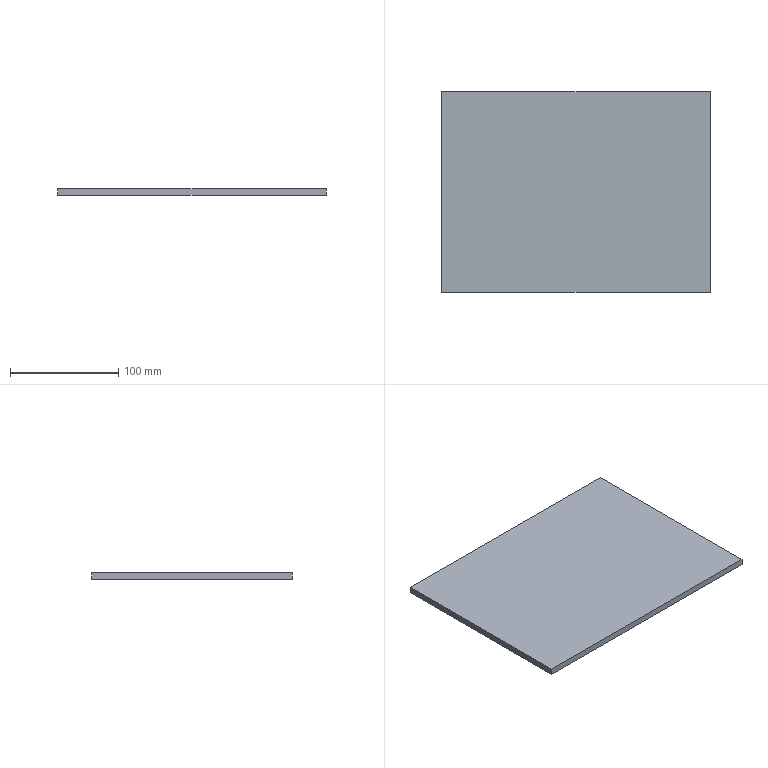Part | SolidWorks | features Extrusion 1 | 1 solid | 6 faces | box 248 x 185 x 6 mm | volume 275280 mm3 | plane 6
STEP:
#1=CARTESIAN_POINT('',(124.,-92.5,0.));
#2=VERTEX_POINT('',#1);
#3=CARTESIAN_POINT('',(124.,92.5,0.));
#4=VERTEX_POINT('',#3);
#5=CARTESIAN_POINT('',(124.,-92.5,0.));
#6=DIRECTION('',(0.,1.,0.));
#7=VECTOR('',#6,1000.);
#8=LINE('',#5,#7);
#9=EDGE_CURVE('',#2,#4,#8,.T.);
#10=ORIENTED_EDGE('',*,*,#9,.T.);
#11=CARTESIAN_POINT('',(124.,92.5,6.));
#12=VERTEX_POINT('',#11);
#13=CARTESIAN_POINT('',(124.,92.5,6.));
#14=DIRECTION('',(0.,0.,-1.));
#15=VECTOR('',#14,1000.);
#16=LINE('',#13,#15);
#17=EDGE_CURVE('',#12,#4,#16,.T.);
#18=ORIENTED_EDGE('',*,*,#17,.F.);
#19=CARTESIAN_POINT('',(124.,-92.5,6.));
#20=VERTEX_POINT('',#19);
#21=CARTESIAN_POINT('',(124.,-92.5,6.));
#22=DIRECTION('',(0.,1.,0.));
#23=VECTOR('',#22,1000.);
#24=LINE('',#21,#23);
#25=EDGE_CURVE('',#20,#12,#24,.T.);
#26=ORIENTED_EDGE('',*,*,#25,.F.);
#27=CARTESIAN_POINT('',(124.,-92.5,6.));
#28=DIRECTION('',(0.,0.,-1.));
#29=VECTOR('',#28,1000.);
#30=LINE('',#27,#29);
#31=EDGE_CURVE('',#20,#2,#30,.T.);
#32=ORIENTED_EDGE('',*,*,#31,.T.);
#33=EDGE_LOOP('',(#10,#18,#26,#32));
#34=FACE_OUTER_BOUND('',#33,.T.);
#35=CARTESIAN_POINT('',(124.,-92.5,6.));
#36=DIRECTION('',(-1.,0.,0.));
#37=DIRECTION('',(0.,0.,1.));
#38=AXIS2_PLACEMENT_3D('',#35,#36,#37);
#39=PLANE('',#38);
#40=ADVANCED_FACE('',(#34),#39,.F.);
#41=CARTESIAN_POINT('',(-124.,92.5,0.));
#42=VERTEX_POINT('',#41);
#43=CARTESIAN_POINT('',(-124.,92.5,0.));
#44=DIRECTION('',(-1.,0.,0.));
#45=VECTOR('',#44,1000.);
#46=LINE('',#43,#45);
#47=EDGE_CURVE('',#4,#42,#46,.T.);
#48=ORIENTED_EDGE('',*,*,#47,.T.);
#49=CARTESIAN_POINT('',(-124.,92.5,6.));
#50=VERTEX_POINT('',#49);
#51=CARTESIAN_POINT('',(-124.,92.5,6.));
#52=DIRECTION('',(0.,0.,-1.));
#53=VECTOR('',#52,1000.);
#54=LINE('',#51,#53);
#55=EDGE_CURVE('',#50,#42,#54,.T.);
#56=ORIENTED_EDGE('',*,*,#55,.F.);
#57=CARTESIAN_POINT('',(-124.,92.5,6.));
#58=DIRECTION('',(-1.,0.,0.));
#59=VECTOR('',#58,1000.);
#60=LINE('',#57,#59);
#61=EDGE_CURVE('',#12,#50,#60,.T.);
#62=ORIENTED_EDGE('',*,*,#61,.F.);
#63=ORIENTED_EDGE('',*,*,#17,.T.);
#64=EDGE_LOOP('',(#48,#56,#62,#63));
#65=FACE_OUTER_BOUND('',#64,.T.);
#66=CARTESIAN_POINT('',(-124.,92.5,6.));
#67=DIRECTION('',(0.,-1.,0.));
#68=DIRECTION('',(0.,0.,-1.));
#69=AXIS2_PLACEMENT_3D('',#66,#67,#68);
#70=PLANE('',#69);
#71=ADVANCED_FACE('',(#65),#70,.F.);
#72=CARTESIAN_POINT('',(-124.,-92.5,0.));
#73=VERTEX_POINT('',#72);
#74=CARTESIAN_POINT('',(-124.,-92.5,0.));
#75=DIRECTION('',(0.,-1.,0.));
#76=VECTOR('',#75,1000.);
#77=LINE('',#74,#76);
#78=EDGE_CURVE('',#42,#73,#77,.T.);
#79=ORIENTED_EDGE('',*,*,#78,.T.);
#80=CARTESIAN_POINT('',(-124.,-92.5,6.));
#81=VERTEX_POINT('',#80);
#82=CARTESIAN_POINT('',(-124.,-92.5,6.));
#83=DIRECTION('',(0.,0.,-1.));
#84=VECTOR('',#83,1000.);
#85=LINE('',#82,#84);
#86=EDGE_CURVE('',#81,#73,#85,.T.);
#87=ORIENTED_EDGE('',*,*,#86,.F.);
#88=CARTESIAN_POINT('',(-124.,-92.5,6.));
#89=DIRECTION('',(0.,-1.,0.));
#90=VECTOR('',#89,1000.);
#91=LINE('',#88,#90);
#92=EDGE_CURVE('',#50,#81,#91,.T.);
#93=ORIENTED_EDGE('',*,*,#92,.F.);
#94=ORIENTED_EDGE('',*,*,#55,.T.);
#95=EDGE_LOOP('',(#79,#87,#93,#94));
#96=FACE_OUTER_BOUND('',#95,.T.);
#97=CARTESIAN_POINT('',(-124.,-92.5,6.));
#98=DIRECTION('',(1.,0.,0.));
#99=DIRECTION('',(0.,0.,-1.));
#100=AXIS2_PLACEMENT_3D('',#97,#98,#99);
#101=PLANE('',#100);
#102=ADVANCED_FACE('',(#96),#101,.F.);
#103=CARTESIAN_POINT('',(-124.,-92.5,0.));
#104=DIRECTION('',(1.,0.,0.));
#105=VECTOR('',#104,1000.);
#106=LINE('',#103,#105);
#107=EDGE_CURVE('',#73,#2,#106,.T.);
#108=ORIENTED_EDGE('',*,*,#107,.T.);
#109=ORIENTED_EDGE('',*,*,#31,.F.);
#110=CARTESIAN_POINT('',(-124.,-92.5,6.));
#111=DIRECTION('',(1.,0.,0.));
#112=VECTOR('',#111,1000.);
#113=LINE('',#110,#112);
#114=EDGE_CURVE('',#81,#20,#113,.T.);
#115=ORIENTED_EDGE('',*,*,#114,.F.);
#116=ORIENTED_EDGE('',*,*,#86,.T.);
#117=EDGE_LOOP('',(#108,#109,#115,#116));
#118=FACE_OUTER_BOUND('',#117,.T.);
#119=CARTESIAN_POINT('',(-124.,-92.5,6.));
#120=DIRECTION('',(0.,1.,0.));
#121=DIRECTION('',(0.,0.,1.));
#122=AXIS2_PLACEMENT_3D('',#119,#120,#121);
#123=PLANE('',#122);
#124=ADVANCED_FACE('',(#118),#123,.F.);
#125=ORIENTED_EDGE('',*,*,#25,.T.);
#126=ORIENTED_EDGE('',*,*,#61,.T.);
#127=ORIENTED_EDGE('',*,*,#92,.T.);
#128=ORIENTED_EDGE('',*,*,#114,.T.);
#129=EDGE_LOOP('',(#125,#126,#127,#128));
#130=FACE_OUTER_BOUND('',#129,.T.);
#131=CARTESIAN_POINT('',(0.,0.,6.));
#132=DIRECTION('',(0.,0.,-1.));
#133=DIRECTION('',(-1.,0.,0.));
#134=AXIS2_PLACEMENT_3D('',#131,#132,#133);
#135=PLANE('',#134);
#136=ADVANCED_FACE('',(#130),#135,.F.);
#137=ORIENTED_EDGE('',*,*,#9,.F.);
#138=ORIENTED_EDGE('',*,*,#107,.F.);
#139=ORIENTED_EDGE('',*,*,#78,.F.);
#140=ORIENTED_EDGE('',*,*,#47,.F.);
#141=EDGE_LOOP('',(#137,#138,#139,#140));
#142=FACE_OUTER_BOUND('',#141,.T.);
#143=CARTESIAN_POINT('',(0.,0.,0.));
#144=DIRECTION('',(0.,0.,-1.));
#145=DIRECTION('',(-1.,0.,0.));
#146=AXIS2_PLACEMENT_3D('',#143,#144,#145);
#147=PLANE('',#146);
#148=ADVANCED_FACE('',(#142),#147,.T.);
#149=CLOSED_SHELL('',(#40,#71,#102,#124,#136,#148));
#150=MANIFOLD_SOLID_BREP('',#149);
#151=CARTESIAN_POINT('',(0.,0.,0.));
#152=DIRECTION('',(0.,0.,1.));
#153=DIRECTION('',(1.,0.,0.));
#154=AXIS2_PLACEMENT_3D('',#151,#152,#153);
#155=(LENGTH_UNIT()NAMED_UNIT(*)SI_UNIT(.MILLI.,.METRE.));
#156=UNCERTAINTY_MEASURE_WITH_UNIT(LENGTH_MEASURE(0.00001),#155,'','');
#157=(NAMED_UNIT(*)PLANE_ANGLE_UNIT()SI_UNIT($,.RADIAN.));
#158=(NAMED_UNIT(*)SI_UNIT($,.STERADIAN.)SOLID_ANGLE_UNIT());
#159=(GEOMETRIC_REPRESENTATION_CONTEXT(3)GLOBAL_UNCERTAINTY_ASSIGNED_CONTEXT((#156))GLOBAL_UNIT_ASSIGNED_CONTEXT((#155,#157,#158))REPRESENTATION_CONTEXT('',''));
#160=ADVANCED_BREP_SHAPE_REPRESENTATION('',(#150,#154),#159);